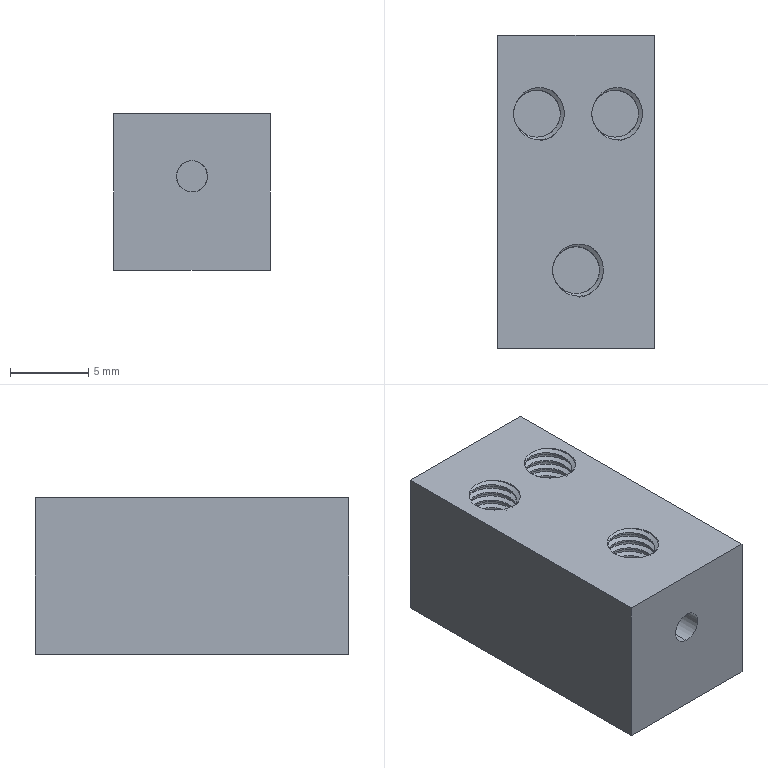Simulation study | abaqus
Set-up summary:
category,name,step,type,value,unit,region
solver,abaqus
solver,version,,,Abaqus/Standard 2020
units,not stated in the deck,,not stated
analysis,deck,,transient,transient
load_step,Step-1,Step-1,transient
load_step,requested,,,1
mesh,nodes,,,2439
mesh,elements,,,2539
element_type,R3D3,,rigid,222
element_type,R3D4,,rigid,2257
element_type,T3D2,,truss,60
load,load commands in deck,,count,3
bc,support commands in deck,,count,21
material,LV,,in results
material,WIRE,,in results
check,setup vs results,,match,"per instance, exact: element labels, types and connectivity; labels of the nodes the elements use; coordinates of those nodes at SINGLE_PRECISION in 4 of 6 instance(s)"
Abaqus input file, long lists of numbers shortened:
*Heading
** Job name: Job-2 Model name: Model-1-Copy
** Generated by: Abaqus/CAE 2020
*Preprint, echo=NO, model=NO, history=NO, contact=NO
**
** PARTS
**
*Part, name=kuai-1
*Node
      1,          10.,           0.,          15.
      2,          10.,         -10.,          15.
** (378 more lines like these left out)
*Element, type=R3D4
 1,   1,   9,  93,  38
 2,   9,  10,  94,  93
** (376 more lines like these left out)
*Node
    381,           0.,           0.,          7.5
*Nset, nset=kuai-1-RefPt_, internal
381,
*Elset, elset=kuai-1, generate
   1,  378,    1
*End Part
**
*Part, name=kuai-2
*Node
      1,          10.,           0.,          20.
      2,          10.,         -10.,          20.
** (250 more lines like these left out)
*Element, type=R3D4
 1,   1,   9,  77,  34
 2,   9,  10,  78,  77
** (248 more lines like these left out)
*Node
    253,          10.,           0.,          10.
*Nset, nset=kuai-2-RefPt_, internal
253,
*Elset, elset=kuai-2, generate
   1,  250,    1
*End Part
**
*Part, name=wire
*Node
      1,   -2.5,   13.114,           0.
      2,   -2.5,  -86.886,           0.
** (62 more lines like these left out)
*Element, type=T3D2
 1,  1, 11
 2, 11, 12
** (58 more lines like these left out)
*Nset, nset=Set-1, generate
  1,  64,   1
*Elset, elset=Set-1, generate
  1,  60,   1
** Section: wirewire
*Solid Section, elset=Set-1, material=wire
1.13,
*End Part
**
*Part, name=work-2
*Node
      1,          19.,       -43.25,          10.
      2,         14.5,       -43.25,          10.
** (625 more lines like these left out)
*Element, type=R3D4
1,   1,  44, 324,  49
2,  44,  45, 325, 324
** (599 more lines like these left out)
*Element, type=R3D3
246,  48, 416,   4
247, 135,  20, 287
** (50 more lines like these left out)
*Node
    628,          9.5,       -38.25,         16.5
*Nset, nset=work-2-RefPt_, internal
628,
*Elset, elset=work-2, generate
   1,  653,    1
*End Part
**
*Part, name=work-3
*Node
      1,           0.,        -225.,           0.
      2,          48.,        -225.,           0.
** (483 more lines like these left out)
*Element, type=R3D4
1,  1, 65, 70,  4
2, 65, 66, 69, 70
** (431 more lines like these left out)
*Element, type=R3D3
152, 391, 307, 387
153, 311, 307, 287
** (106 more lines like these left out)
*Node
    486,          48.,       -112.5,           0.
*Nset, nset=work-3-RefPt_, internal
486,
*Elset, elset=work-3, generate
   1,  541,    1
*End Part
**
*Part, name=work-4
*Node
      1,         33.5,       -43.25,          10.
      2,          29.,       -43.25,          10.
** (624 more lines like these left out)
*Element, type=R3D4
1,   1,  46, 325,  51
2,  46,  47, 326, 325
** (593 more lines like these left out)
*Element, type=R3D3
246, 452, 451, 439
247, 146,  28, 287
** (60 more lines like these left out)
*Node
    627,         38.5,       -38.25,         16.5
*Nset, nset=work-4-RefPt_, internal
627,
*Elset, elset=work-4, generate
   1,  657,    1
*End Part
**
**
** ASSEMBLY
**
*Assembly, name=Assembly
**
*Instance, name=work-2-1, part=work-2
*End Instance
**
*Instance, name=work-4-1, part=work-4
*End Instance
**
*Instance, name=work-3-1, part=work-3
*End Instance
**
*Instance, name=kuai-1-1, part=kuai-1
         19.,        -200.,           5.
*End Instance
**
*Instance, name=kuai-2-1, part=kuai-2
         19.,         -80.,          20.
         19.,         -80.,          20., 20.,         -80.,          20., 90.
*End Instance
**
*Instance, name=wire-1, part=wire
   24.,  -113.114,          15.
*End Instance
**
*Nset, nset=Set-6, instance=work-3-1
 486,
*Nset, nset=Set-12, instance=wire-1
  2, 10
*Nset, nset=Set-13, instance=kuai-1-1, generate
   1,  344,    1
*Elset, elset=Set-13, instance=kuai-1-1, generate
   1,  329,    1
*Nset, nset=Set-14, instance=kuai-2-1
   1,   2,   3,   4,   5,   6,   7,   8,   9,  10,  11,  12,  13,  14,  15,  16
  17,  18,  19,  20,  21,  22,  23,  24,  25,  26,  27,  28,  29,  30,  31,  32
** (12 more lines like these left out)
*Elset, elset=Set-14, instance=kuai-2-1
   1,   2,   3,   4,   5,   6,   7,   8,   9,  10,  11,  12,  13,  14,  15,  16
  17,  18,  19,  20,  21,  22,  23,  24,  25,  26,  27,  28,  29,  30,  31,  32
** (11 more lines like these left out)
*Nset, nset=Set-17, instance=kuai-2-1
 253,
*Nset, nset=Set-18, instance=kuai-1-1
 381,
*Nset, nset=Set-19, instance=kuai-1-1
 381,
*Nset, nset=Set-20, instance=work-3-1
 486,
*Nset, nset=Set-21, instance=kuai-1-1
 381,
*Nset, nset=Set-22, instance=wire-1
  2, 10
*Nset, nset=Set-23, instance=work-2-1
 628,
*Nset, nset=Set-23, instance=work-4-1
 627,
*Nset, nset=Set-40, instance=work-2-1
 628,
*Nset, nset=Set-41, instance=work-4-1
 627,
*Nset, nset=m_Set-8, instance=wire-1
  3,  4, 30, 31
*Elset, elset=m_Set-8, instance=wire-1, generate
 21,  23,   1
*Nset, nset=m_Set-9, instance=wire-1
  6,  7, 38, 39
*Elset, elset=m_Set-9, instance=wire-1, generate
 31,  33,   1
*Nset, nset=m_Set-10, instance=wire-1
 5, 8
*Nset, nset=m_Set-11, instance=wire-1
 1, 9
*Nset, nset=m_Set-15, instance=wire-1
 3,
*Nset, nset=m_Set-16, instance=wire-1
 6,
*Nset, nset=m_Set-30, instance=work-2-1
 628,
*Nset, nset=m_Set-32, instance=work-4-1
 627,
*Nset, nset=m_Set-34, instance=work-2-1
  11,  12,  13,  14,  15,  16,  75,  76,  77,  78,  79,  80,  81,  82,  83,  84
  85,  86,  87,  88,  89,  90,  91,  92,  93,  94,  95,  96,  97,  98,  99, 100
** (2 more lines like these left out)
*Elset, elset=m_Set-34, instance=work-2-1, generate
 33,  72,   1
*Nset, nset=m_Set-36, instance=work-4-1
  10,  11,  14,  15,  16,  17,  58,  59,  60,  61,  62,  63,  64,  65,  66,  67
  68,  69,  70,  71,  72,  73,  74,  75,  76,  95,  96,  97,  98,  99, 100, 101
** (2 more lines like these left out)
*Elset, elset=m_Set-36, instance=work-4-1, generate
 33,  72,   1
*Nset, nset=s_Set-24, instance=wire-1
 3,
*Nset, nset=s_Set-25, instance=wire-1
 6,
*Nset, nset=s_Set-26, instance=wire-1
 5, 8
*Nset, nset=s_Set-27, instance=wire-1
 1, 9
*Nset, nset=s_Set-28, instance=wire-1
  3,  4, 30, 31
*Elset, elset=s_Set-28, instance=wire-1, generate
 21,  23,   1
*Nset, nset=s_Set-29, instance=wire-1
  6,  7, 38, 39
*Elset, elset=s_Set-29, instance=wire-1, generate
 31,  33,   1
*Nset, nset=s_Set-30, instance=wire-1
  3,  4, 30, 31
*Elset, elset=s_Set-30, instance=wire-1, generate
 21,  23,   1
*Nset, nset=s_Set-32, instance=wire-1
  6,  7, 38, 39
*Elset, elset=s_Set-32, instance=wire-1, generate
 31,  33,   1
*Nset, nset=s_Set-34, instance=wire-1
 3,
*Nset, nset=s_Set-36, instance=wire-1
 6,
*Nset, nset=s_Set-38, instance=wire-1
 6,
*Nset, nset=s_Set-39, instance=wire-1
 3,
*Elset, elset=_m_Surf-5_SPOS, internal, instance=work-2-1, generate
 33,  72,   1
*Surface, type=ELEMENT, name=m_Surf-5
_m_Surf-5_SPOS, SPOS
*Elset, elset=_m_Surf-6_SPOS, internal, instance=work-4-1, generate
 33,  72,   1
*Surface, type=ELEMENT, name=m_Surf-6
_m_Surf-6_SPOS, SPOS
*Elset, elset=_m_Surf-7_SPOS, internal, instance=kuai-2-1, generate
 226,  250,    1
*Surface, type=ELEMENT, name=m_Surf-7
_m_Surf-7_SPOS, SPOS
*Elset, elset=_m_Surf-8_SPOS, internal, instance=kuai-2-1, generate
 201,  225,    1
*Surface, type=ELEMENT, name=m_Surf-8
_m_Surf-8_SPOS, SPOS
*Elset, elset=_m_Surf-11_SNEG, internal, instance=work-4-1, generate
 33,  72,   1
*Surface, type=ELEMENT, name=m_Surf-11
_m_Surf-11_SNEG, SNEG
*Elset, elset=_m_Surf-12_SNEG, internal, instance=work-2-1, generate
 33,  72,   1
*Surface, type=ELEMENT, name=m_Surf-12
_m_Surf-12_SNEG, SNEG
*Elset, elset=_s_Surf-1_SPOS, internal, instance=work-2-1, generate
 33,  72,   1
*Surface, type=ELEMENT, name=s_Surf-1
_s_Surf-1_SPOS, SPOS
*Elset, elset=_s_Surf-2_SPOS, internal, instance=work-4-1, generate
 33,  72,   1
*Surface, type=ELEMENT, name=s_Surf-2
_s_Surf-2_SPOS, SPOS
*Elset, elset=_s_Surf-3_SPOS, internal, instance=kuai-2-1, generate
 226,  250,    1
*Surface, type=ELEMENT, name=s_Surf-3
_s_Surf-3_SPOS, SPOS
*Elset, elset=_s_Surf-4_SPOS, internal, instance=kuai-2-1, generate
 201,  225,    1
*Surface, type=ELEMENT, name=s_Surf-4
_s_Surf-4_SPOS, SPOS
*Elset, elset=_s_Surf-9_, internal, instance=wire-1, generate
 21,  23,   1
*Surface, type=ELEMENT, name=s_Surf-9
_s_Surf-9_,
*Elset, elset=_s_Surf-10_, internal, instance=wire-1, generate
 31,  33,   1
*Surface, type=ELEMENT, name=s_Surf-10
_s_Surf-10_,
*Surface, type=NODE, name=s_Set-38_CNS_, internal
s_Set-38, 1.
*Surface, type=NODE, name=s_Set-39_CNS_, internal
s_Set-39, 1.
*Surface, type=NODE, name=s_Set-26_CNS_, internal
s_Set-26, 1.
*Surface, type=NODE, name=s_Set-27_CNS_, internal
s_Set-27, 1.
*Rigid Body, ref node=work-2-1.work-2-RefPt_, elset=work-2-1.work-2
*Rigid Body, ref node=work-4-1.work-4-RefPt_, elset=work-4-1.work-4
*Rigid Body, ref node=work-3-1.work-3-RefPt_, elset=work-3-1.work-3
*Rigid Body, ref node=kuai-1-1.kuai-1-RefPt_, elset=kuai-1-1.kuai-1
*Rigid Body, ref node=kuai-2-1.kuai-2-RefPt_, elset=kuai-2-1.kuai-2
** Constraint: Constraint-1
*Tie, name=Constraint-1, adjust=yes
s_Set-38_CNS_, m_Surf-11
** Constraint: Constraint-2
*Tie, name=Constraint-2, adjust=yes
s_Set-39_CNS_, m_Surf-12
** Constraint: Constraint-3
*Tie, name=Constraint-3, adjust=yes
s_Set-26_CNS_, m_Surf-7
** Constraint: Constraint-4
*Tie, name=Constraint-4, adjust=yes
s_Set-27_CNS_, m_Surf-8
*Elset, elset=__Int-1_gcs0_6_SPOS, internal, instance=work-2-1, generate
 33,  72,   1
*Surface, type=ELEMENT, name=_Int-1_gcs0_6, internal
__Int-1_gcs0_6_SPOS, SPOS
*Elset, elset=__Int-1_gcs0_12_SPOS, internal, instance=work-2-1, generate
 111,  119,    1
*Surface, type=ELEMENT, name=_Int-1_gcs0_12, internal
__Int-1_gcs0_12_SPOS, SPOS
*Elset, elset=__Int-1_gcs0_22_SPOS, internal, instance=work-2-1, generate
 589,  653,    1
*Surface, type=ELEMENT, name=_Int-1_gcs0_22, internal
__Int-1_gcs0_22_SPOS, SPOS
*Elset, elset=__Int-1_gcs0_23_SPOS, internal, instance=work-2-1, generate
 222,  237,    1
*Surface, type=ELEMENT, name=_Int-1_gcs0_23, internal
__Int-1_gcs0_23_SPOS, SPOS
*Elset, elset=__Int-1_gcs0_24_SPOS, internal, instance=work-2-1, generate
 238,  245,    1
*Surface, type=ELEMENT, name=_Int-1_gcs0_24, internal
__Int-1_gcs0_24_SPOS, SPOS
*Elset, elset=__Int-1_gcs0_30_SNEG, internal, instance=work-2-1, generate
 33,  72,   1
*Surface, type=ELEMENT, name=_Int-1_gcs0_30, internal
__Int-1_gcs0_30_SNEG, SNEG
*Elset, elset=__Int-1_gcs0_36_SNEG, internal, instance=work-2-1, generate
 111,  119,    1
*Surface, type=ELEMENT, name=_Int-1_gcs0_36, internal
__Int-1_gcs0_36_SNEG, SNEG
*Elset, elset=__Int-1_gcs0_46_SNEG, internal, instance=work-2-1, generate
 589,  653,    1
*Surface, type=ELEMENT, name=_Int-1_gcs0_46, internal
__Int-1_gcs0_46_SNEG, SNEG
*Elset, elset=__Int-1_gcs0_47_SNEG, internal, instance=work-2-1, generate
 222,  237,    1
*Surface, type=ELEMENT, name=_Int-1_gcs0_47, internal
__Int-1_gcs0_47_SNEG, SNEG
*Elset, elset=__Int-1_gcs0_48_SNEG, internal, instance=work-2-1, generate
 238,  245,    1
*Surface, type=ELEMENT, name=_Int-1_gcs0_48, internal
__Int-1_gcs0_48_SNEG, SNEG
*Elset, elset=__Int-1_gcs0_54_SPOS, internal, instance=work-4-1, generate
 33,  72,   1
*Surface, type=ELEMENT, name=_Int-1_gcs0_54, internal
__Int-1_gcs0_54_SPOS, SPOS
*Elset, elset=__Int-1_gcs0_60_SPOS, internal, instance=work-4-1, generate
 111,  119,    1
*Surface, type=ELEMENT, name=_Int-1_gcs0_60, internal
__Int-1_gcs0_60_SPOS, SPOS
*Elset, elset=__Int-1_gcs0_70_SPOS, internal, instance=work-4-1, generate
 595,  657,    1
*Surface, type=ELEMENT, name=_Int-1_gcs0_70, internal
__Int-1_gcs0_70_SPOS, SPOS
*Elset, elset=__Int-1_gcs0_71_SPOS, internal, instance=work-4-1, generate
 222,  237,    1
*Surface, type=ELEMENT, name=_Int-1_gcs0_71, internal
__Int-1_gcs0_71_SPOS, SPOS
*Elset, elset=__Int-1_gcs0_72_SPOS, internal, instance=work-4-1, generate
 238,  245,    1
*Surface, type=ELEMENT, name=_Int-1_gcs0_72, internal
__Int-1_gcs0_72_SPOS, SPOS
*Elset, elset=__Int-1_gcs0_78_SNEG, internal, instance=work-4-1, generate
 33,  72,   1
*Surface, type=ELEMENT, name=_Int-1_gcs0_78, internal
__Int-1_gcs0_78_SNEG, SNEG
*Elset, elset=__Int-1_gcs0_84_SNEG, internal, instance=work-4-1, generate
 111,  119,    1
*Surface, type=ELEMENT, name=_Int-1_gcs0_84, internal
__Int-1_gcs0_84_SNEG, SNEG
*Elset, elset=__Int-1_gcs0_94_SNEG, internal, instance=work-4-1, generate
 595,  657,    1
*Surface, type=ELEMENT, name=_Int-1_gcs0_94, internal
__Int-1_gcs0_94_SNEG, SNEG
*Elset, elset=__Int-1_gcs0_95_SNEG, internal, instance=work-4-1, generate
 222,  237,    1
*Surface, type=ELEMENT, name=_Int-1_gcs0_95, internal
__Int-1_gcs0_95_SNEG, SNEG
*Elset, elset=__Int-1_gcs0_96_SNEG, internal, instance=work-4-1, generate
 238,  245,    1
*Surface, type=ELEMENT, name=_Int-1_gcs0_96, internal
__Int-1_gcs0_96_SNEG, SNEG
*Elset, elset=__Int-1_gcs0_103_SPOS, internal, instance=work-3-1, generate
 89,  95,   1
*Surface, type=ELEMENT, name=_Int-1_gcs0_103, internal
__Int-1_gcs0_103_SPOS, SPOS
*Elset, elset=__Int-1_gcs0_105_SPOS, internal, instance=work-3-1, generate
  96,  102,    1
*Surface, type=ELEMENT, name=_Int-1_gcs0_105, internal
__Int-1_gcs0_105_SPOS, SPOS
*Elset, elset=__Int-1_gcs0_128_SPOS, internal, instance=work-3-1, generate
 124,  131,    1
*Surface, type=ELEMENT, name=_Int-1_gcs0_128, internal
__Int-1_gcs0_128_SPOS, SPOS
*Elset, elset=__Int-1_gcs0_129_SPOS, internal, instance=work-3-1, generate
 132,  139,    1
*Surface, type=ELEMENT, name=_Int-1_gcs0_129, internal
__Int-1_gcs0_129_SPOS, SPOS
*Elset, elset=__Int-1_gcs0_130_SPOS, internal, instance=work-3-1, generate
 140,  145,    1
*Surface, type=ELEMENT, name=_Int-1_gcs0_130, internal
__Int-1_gcs0_130_SPOS, SPOS
*Elset, elset=__Int-1_gcs0_131_SPOS, internal, instance=work-3-1, generate
 146,  151,    1
*Surface, type=ELEMENT, name=_Int-1_gcs0_131, internal
__Int-1_gcs0_131_SPOS, SPOS
*Elset, elset=__Int-1_gcs0_138_SNEG, internal, instance=work-3-1, generate
 89,  95,   1
*Surface, type=ELEMENT, name=_Int-1_gcs0_138, internal
__Int-1_gcs0_138_SNEG, SNEG
*Elset, elset=__Int-1_gcs0_140_SNEG, internal, instance=work-3-1, generate
  96,  102,    1
*Surface, type=ELEMENT, name=_Int-1_gcs0_140, internal
__Int-1_gcs0_140_SNEG, SNEG
*Elset, elset=__Int-1_gcs0_163_SNEG, internal, instance=work-3-1, generate
 124,  131,    1
*Surface, type=ELEMENT, name=_Int-1_gcs0_163, internal
__Int-1_gcs0_163_SNEG, SNEG
*Elset, elset=__Int-1_gcs0_164_SNEG, internal, instance=work-3-1, generate
 132,  139,    1
*Surface, type=ELEMENT, name=_Int-1_gcs0_164, internal
__Int-1_gcs0_164_SNEG, SNEG
*Elset, elset=__Int-1_gcs0_165_SNEG, internal, instance=work-3-1, generate
 140,  145,    1
*Surface, type=ELEMENT, name=_Int-1_gcs0_165, internal
__Int-1_gcs0_165_SNEG, SNEG
*Elset, elset=__Int-1_gcs0_166_SNEG, internal, instance=work-3-1, generate
 146,  151,    1
*Surface, type=ELEMENT, name=_Int-1_gcs0_166, internal
__Int-1_gcs0_166_SNEG, SNEG
*End Assembly
*Amplitude, name=Amp-1
             0.,              0.,              1.,              1.
**
** MATERIALS
**
*Material, name=lv
*Density
 2.7e-09,
*Elastic
78000., 0.35
*Material, name=wire
*Density
 7.8e-09,
*Elastic
1700., 0.4
**
** INTERACTION PROPERTIES
**
*Surface Interaction, name=IntProp-1
1.,
*Friction
0.,
*Surface Behavior, pressure-overclosure=HARD
**
** INTERACTIONS
**
** Interaction: Int-1
*Contact
*Contact Inclusions, ALL EXTERIOR
*Contact Property Assignment
 ,  , IntProp-1
*Surface Property Assignment, property=GEOMETRIC CORRECTION
_Int-1_gcs0_6, Circumferential, 9.5, -38.25, 15.5,  9.5, -38.25, 14.5
_Int-1_gcs0_12, Circumferential, 9.5, -38.25, 10.5,  9.5, -38.25, 9.5
_Int-1_gcs0_22, Circumferential, 9.5, -38.25, 16.5,  9.5, -38.25, 15.5
_Int-1_gcs0_23, Circumferential, 9.5, -38.25, 7.,  9.5, -38.25, 8.
_Int-1_gcs0_24, Circumferential, 10.25, -42.579, 15.,  9.25, -42.579, 15.
_Int-1_gcs0_30, Circumferential, 9.5, -38.25, 15.5,  9.5, -38.25, 14.5
_Int-1_gcs0_36, Circumferential, 9.5, -38.25, 10.5,  9.5, -38.25, 9.5
_Int-1_gcs0_46, Circumferential, 9.5, -38.25, 16.5,  9.5, -38.25, 15.5
_Int-1_gcs0_47, Circumferential, 9.5, -38.25, 7.,  9.5, -38.25, 8.
_Int-1_gcs0_48, Circumferential, 10.25, -42.579, 15.,  9.25, -42.579, 15.
_Int-1_gcs0_54, Circumferential, 38.5, -38.25, 15.5,  38.5, -38.25, 14.5
_Int-1_gcs0_60, Circumferential, 38.5, -38.25, 10.5,  38.5, -38.25, 9.5
_Int-1_gcs0_70, Circumferential, 38.5, -38.25, 16.5,  38.5, -38.25, 15.5
_Int-1_gcs0_71, Circumferential, 38.5, -38.25, 7.,  38.5, -38.25, 8.
_Int-1_gcs0_72, Circumferential, 37.75, -42.579, 15.,  38.75, -42.579, 15.
_Int-1_gcs0_78, Circumferential, 38.5, -38.25, 15.5,  38.5, -38.25, 14.5
_Int-1_gcs0_84, Circumferential, 38.5, -38.25, 10.5,  38.5, -38.25, 9.5
_Int-1_gcs0_94, Circumferential, 38.5, -38.25, 16.5,  38.5, -38.25, 15.5
_Int-1_gcs0_95, Circumferential, 38.5, -38.25, 7.,  38.5, -38.25, 8.
_Int-1_gcs0_96, Circumferential, 37.75, -42.579, 15.,  38.75, -42.579, 15.
_Int-1_gcs0_103, Circumferential, 38.5, -38.25, 10.,  38.5, -38.25, 9.
_Int-1_gcs0_105, Circumferential, 9.5, -38.25, 10.,  9.5, -38.25, 9.
_Int-1_gcs0_128, Circumferential, 38.5, -38.25, 8.,  38.5, -38.25, 7.
_Int-1_gcs0_129, Circumferential, 9.5, -38.25, 8.,  9.5, -38.25, 7.
_Int-1_gcs0_130, Circumferential, 21.5, -52.5, 15.,  21.5, -51.5, 15.
_Int-1_gcs0_131, Circumferential, 26.5, -52.5, 15.,  26.5, -51.5, 15.
_Int-1_gcs0_138, Circumferential, 38.5, -38.25, 10.,  38.5, -38.25, 9.
_Int-1_gcs0_140, Circumferential, 9.5, -38.25, 10.,  9.5, -38.25, 9.
_Int-1_gcs0_163, Circumferential, 38.5, -38.25, 8.,  38.5, -38.25, 7.
_Int-1_gcs0_164, Circumferential, 9.5, -38.25, 8.,  9.5, -38.25, 7.
_Int-1_gcs0_165, Circumferential, 21.5, -52.5, 15.,  21.5, -51.5, 15.
_Int-1_gcs0_166, Circumferential, 26.5, -52.5, 15.,  26.5, -51.5, 15.
** ----------------------------------------------------------------
**
** STEP: Step-1
**
*Step, name=Step-1, nlgeom=YES, inc=1000
*Dynamic
0.001,1.,1e-05
**
** BOUNDARY CONDITIONS
**
** Name: BC-1 Type: 对称/反对称/完全固定
*Boundary
Set-21, ENCASTRE
** Name: BC-2 Type: 对称/反对称/完全固定
*Boundary
Set-6, ENCASTRE
** Name: BC-3 Type: 位移/转角
*Boundary, amplitude=Amp-1
Set-17, 1, 1
Set-17, 2, 2, -10.
Set-17, 3, 3
Set-17, 4, 4
Set-17, 5, 5
Set-17, 6, 6
** Name: BC-4 Type: 对称/反对称/完全固定
*Boundary
Set-22, ENCASTRE
** Name: BC-5 Type: 位移/转角
*Boundary, amplitude=Amp-1
Set-40, 1, 1
Set-40, 2, 2
Set-40, 3, 3
Set-40, 4, 4
Set-40, 5, 5
Set-40, 6, 6, -1.55
** Name: BC-5-Copy Type: 位移/转角
*Boundary, amplitude=Amp-1
Set-41, 1, 1
Set-41, 2, 2
Set-41, 3, 3
Set-41, 4, 4
Set-41, 5, 5
Set-41, 6, 6, 1.55
**
** OUTPUT REQUESTS
**
*Restart, write, number interval=1, time marks=NO
**
** FIELD OUTPUT: F-Output-1
**
*Output, field, frequency=1
*Node Output
CF, RF, RT, U, V
*Element Output, directions=YES
E, LE, MISES, PE, PEEQ, PEMAG, S, SF
*Contact Output
CDISP, CSTRESS
**
** HISTORY OUTPUT: H-Output-1
**
*Output, history, variable=PRESELECT, frequency=1
*End Step
Results summary:
result,step,,partial,increments=229 time=0.05152/1.0
result,analysis,,,transient
result,last_loadstep,,,1
result,primary field,,,U
result,reaction total,,FX,0.003418,model units
result,reaction total,,FY,4.1e-05,model units
result,reaction total,,FZ,2.9e-05,model units